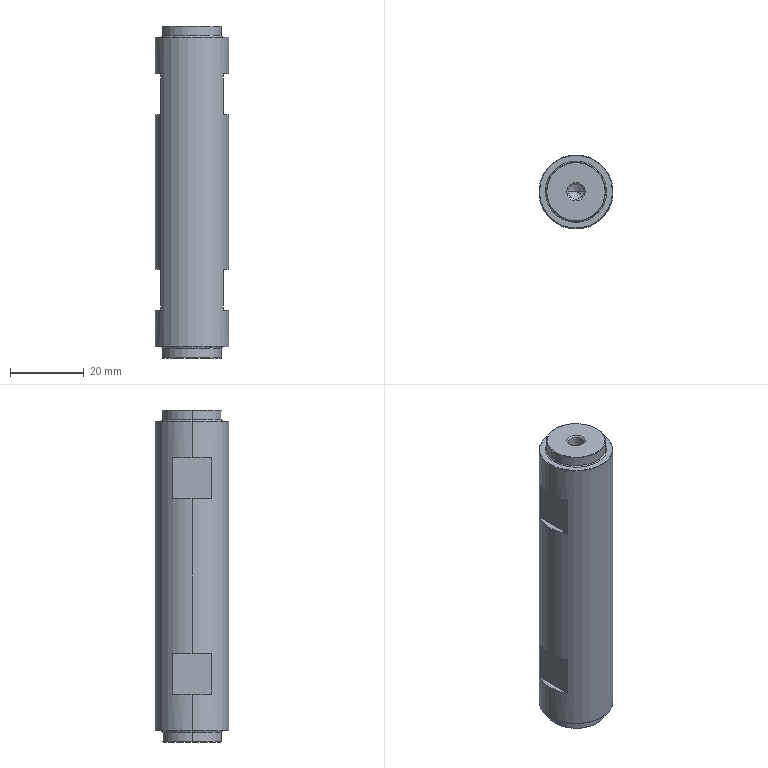Part | SolidWorks | features BaseBody 1 | 1 solid | 46 faces | box 20 x 20 x 90 mm | volume 26843 mm3 | cone 16 | plane 16 | cylinder 10 | spline 4 | commonest cylinder face diameters 4.134 x4 16 x4 20 x2
STEP:
#1=CARTESIAN_POINT('',(8.,0.,-2.7));
#2=VERTEX_POINT('',#1);
#3=CARTESIAN_POINT('',(-8.,0.,-2.7));
#4=VERTEX_POINT('',#3);
#5=CARTESIAN_POINT('',(0.,0.,-2.7));
#6=DIRECTION('',(0.,0.,1.));
#7=DIRECTION('',(-1.,0.,0.));
#8=AXIS2_PLACEMENT_3D('',#5,#6,#7);
#9=CIRCLE('',#8,8.);
#10=EDGE_CURVE('',#2,#4,#9,.T.);
#11=ORIENTED_EDGE('',*,*,#10,.F.);
#12=CARTESIAN_POINT('',(8.3,0.,-3.));
#13=VERTEX_POINT('',#12);
#14=CARTESIAN_POINT('',(8.3,0.,-2.7));
#15=DIRECTION('',(0.,-1.,0.));
#16=DIRECTION('',(1.,0.,0.));
#17=AXIS2_PLACEMENT_3D('',#14,#15,#16);
#18=CIRCLE('',#17,0.3);
#19=EDGE_CURVE('',#2,#13,#18,.T.);
#20=ORIENTED_EDGE('',*,*,#19,.T.);
#21=CARTESIAN_POINT('',(-8.3,0.,-3.));
#22=VERTEX_POINT('',#21);
#23=CARTESIAN_POINT('',(8.3,0.,-3.));
#24=CARTESIAN_POINT('',(8.3,16.6,-3.));
#25=CARTESIAN_POINT('',(-8.3,16.6,-3.));
#26=CARTESIAN_POINT('',(-8.3,0.,-3.));
#27=(BOUNDED_CURVE()B_SPLINE_CURVE(3,(#23,#24,#25,#26),.UNSPECIFIED.,.F.,.F.)B_SPLINE_CURVE_WITH_KNOTS((4,4),(0.5,1.),.UNSPECIFIED.)CURVE()GEOMETRIC_REPRESENTATION_ITEM()RATIONAL_B_SPLINE_CURVE((1.,0.3333,0.3333,1.))REPRESENTATION_ITEM(''));
#28=EDGE_CURVE('',#13,#22,#27,.T.);
#29=ORIENTED_EDGE('',*,*,#28,.T.);
#30=CARTESIAN_POINT('',(-8.3,0.,-2.7));
#31=DIRECTION('',(0.,1.,0.));
#32=DIRECTION('',(-1.,0.,0.));
#33=AXIS2_PLACEMENT_3D('',#30,#31,#32);
#34=CIRCLE('',#33,0.3);
#35=EDGE_CURVE('',#4,#22,#34,.T.);
#36=ORIENTED_EDGE('',*,*,#35,.F.);
#37=EDGE_LOOP('',(#11,#20,#29,#36));
#38=FACE_OUTER_BOUND('',#37,.T.);
#39=CARTESIAN_POINT('',(-8.,0.,-2.7));
#40=CARTESIAN_POINT('',(-8.,16.,-2.7));
#41=CARTESIAN_POINT('',(8.,16.,-2.7));
#42=CARTESIAN_POINT('',(8.,0.,-2.7));
#43=CARTESIAN_POINT('',(-8.,0.,-2.876));
#44=CARTESIAN_POINT('',(-8.,16.,-2.876));
#45=CARTESIAN_POINT('',(8.,16.,-2.876));
#46=CARTESIAN_POINT('',(8.,0.,-2.876));
#47=CARTESIAN_POINT('',(-8.124,0.,-3.));
#48=CARTESIAN_POINT('',(-8.124,16.249,-3.));
#49=CARTESIAN_POINT('',(8.124,16.249,-3.));
#50=CARTESIAN_POINT('',(8.124,0.,-3.));
#51=CARTESIAN_POINT('',(-8.3,0.,-3.));
#52=CARTESIAN_POINT('',(-8.3,16.6,-3.));
#53=CARTESIAN_POINT('',(8.3,16.6,-3.));
#54=CARTESIAN_POINT('',(8.3,0.,-3.));
#55=(BOUNDED_SURFACE()B_SPLINE_SURFACE(3,3,((#39,#40,#41,#42),(#43,#44,#45,#46),(#47,#48,#49,#50),(#51,#52,#53,#54)),.UNSPECIFIED.,.F.,.F.,.F.)B_SPLINE_SURFACE_WITH_KNOTS((4,4),(4,4),(0.,1.),(0.,1.),.UNSPECIFIED.)GEOMETRIC_REPRESENTATION_ITEM()RATIONAL_B_SPLINE_SURFACE(((1.,0.3333,0.3333,1.),(0.8047,0.2682,0.2682,0.8047),(0.8047,0.2682,0.2682,0.8047),(1.,0.3333,0.3333,1.)))REPRESENTATION_ITEM('')SURFACE());
#56=ADVANCED_FACE('',(#38),#55,.F.);
#57=CARTESIAN_POINT('',(-8.3,0.,-87.));
#58=VERTEX_POINT('',#57);
#59=CARTESIAN_POINT('',(8.3,0.,-87.));
#60=VERTEX_POINT('',#59);
#61=CARTESIAN_POINT('',(-8.3,0.,-87.));
#62=CARTESIAN_POINT('',(-8.3,16.6,-87.));
#63=CARTESIAN_POINT('',(8.3,16.6,-87.));
#64=CARTESIAN_POINT('',(8.3,0.,-87.));
#65=(BOUNDED_CURVE()B_SPLINE_CURVE(3,(#61,#62,#63,#64),.UNSPECIFIED.,.F.,.T.)B_SPLINE_CURVE_WITH_KNOTS((4,4),(0.,0.5),.UNSPECIFIED.)CURVE()GEOMETRIC_REPRESENTATION_ITEM()RATIONAL_B_SPLINE_CURVE((1.,0.3333,0.3333,1.))REPRESENTATION_ITEM(''));
#66=EDGE_CURVE('',#58,#60,#65,.T.);
#67=ORIENTED_EDGE('',*,*,#66,.T.);
#68=CARTESIAN_POINT('',(8.,0.,-87.3));
#69=VERTEX_POINT('',#68);
#70=CARTESIAN_POINT('',(8.3,0.,-87.3));
#71=DIRECTION('',(0.,-1.,0.));
#72=DIRECTION('',(1.,0.,0.));
#73=AXIS2_PLACEMENT_3D('',#70,#71,#72);
#74=CIRCLE('',#73,0.3);
#75=EDGE_CURVE('',#60,#69,#74,.T.);
#76=ORIENTED_EDGE('',*,*,#75,.T.);
#77=CARTESIAN_POINT('',(-8.,0.,-87.3));
#78=VERTEX_POINT('',#77);
#79=CARTESIAN_POINT('',(0.,0.,-87.3));
#80=DIRECTION('',(0.,0.,-1.));
#81=DIRECTION('',(-1.,0.,0.));
#82=AXIS2_PLACEMENT_3D('',#79,#80,#81);
#83=CIRCLE('',#82,8.);
#84=EDGE_CURVE('',#78,#69,#83,.T.);
#85=ORIENTED_EDGE('',*,*,#84,.F.);
#86=CARTESIAN_POINT('',(-8.3,0.,-87.3));
#87=DIRECTION('',(0.,1.,0.));
#88=DIRECTION('',(-1.,0.,0.));
#89=AXIS2_PLACEMENT_3D('',#86,#87,#88);
#90=CIRCLE('',#89,0.3);
#91=EDGE_CURVE('',#58,#78,#90,.T.);
#92=ORIENTED_EDGE('',*,*,#91,.F.);
#93=EDGE_LOOP('',(#67,#76,#85,#92));
#94=FACE_OUTER_BOUND('',#93,.T.);
#95=CARTESIAN_POINT('',(-8.3,0.,-87.));
#96=CARTESIAN_POINT('',(-8.3,16.6,-87.));
#97=CARTESIAN_POINT('',(8.3,16.6,-87.));
#98=CARTESIAN_POINT('',(8.3,0.,-87.));
#99=CARTESIAN_POINT('',(-8.124,0.,-87.));
#100=CARTESIAN_POINT('',(-8.124,16.249,-87.));
#101=CARTESIAN_POINT('',(8.124,16.249,-87.));
#102=CARTESIAN_POINT('',(8.124,0.,-87.));
#103=CARTESIAN_POINT('',(-8.,0.,-87.124));
#104=CARTESIAN_POINT('',(-8.,16.,-87.124));
#105=CARTESIAN_POINT('',(8.,16.,-87.124));
#106=CARTESIAN_POINT('',(8.,0.,-87.124));
#107=CARTESIAN_POINT('',(-8.,0.,-87.3));
#108=CARTESIAN_POINT('',(-8.,16.,-87.3));
#109=CARTESIAN_POINT('',(8.,16.,-87.3));
#110=CARTESIAN_POINT('',(8.,0.,-87.3));
#111=(BOUNDED_SURFACE()B_SPLINE_SURFACE(3,3,((#95,#96,#97,#98),(#99,#100,#101,#102),(#103,#104,#105,#106),(#107,#108,#109,#110)),.UNSPECIFIED.,.F.,.F.,.F.)B_SPLINE_SURFACE_WITH_KNOTS((4,4),(4,4),(0.,1.),(0.,1.),.UNSPECIFIED.)GEOMETRIC_REPRESENTATION_ITEM()RATIONAL_B_SPLINE_SURFACE(((1.,0.3333,0.3333,1.),(0.8047,0.2682,0.2682,0.8047),(0.8047,0.2682,0.2682,0.8047),(1.,0.3333,0.3333,1.)))REPRESENTATION_ITEM('')SURFACE());
#112=ADVANCED_FACE('',(#94),#111,.F.);
#113=CARTESIAN_POINT('',(10.,0.,-86.9));
#114=VERTEX_POINT('',#113);
#115=CARTESIAN_POINT('',(-10.,0.,-86.9));
#116=VERTEX_POINT('',#115);
#117=CARTESIAN_POINT('',(0.,0.,-86.9));
#118=DIRECTION('',(0.,0.,1.));
#119=DIRECTION('',(1.,0.,0.));
#120=AXIS2_PLACEMENT_3D('',#117,#118,#119);
#121=CIRCLE('',#120,10.);
#122=EDGE_CURVE('',#114,#116,#121,.T.);
#123=ORIENTED_EDGE('',*,*,#122,.T.);
#124=CARTESIAN_POINT('',(-10.,0.,-77.));
#125=VERTEX_POINT('',#124);
#126=CARTESIAN_POINT('',(-10.,0.,-90.));
#127=DIRECTION('',(0.,0.,1.));
#128=VECTOR('',#127,1000.);
#129=LINE('',#126,#128);
#130=EDGE_CURVE('',#116,#125,#129,.T.);
#131=ORIENTED_EDGE('',*,*,#130,.T.);
#132=CARTESIAN_POINT('',(-8.5,5.268,-77.));
#133=VERTEX_POINT('',#132);
#134=CARTESIAN_POINT('',(0.,0.,-77.));
#135=DIRECTION('',(0.,0.,-1.));
#136=DIRECTION('',(1.,0.,0.));
#137=AXIS2_PLACEMENT_3D('',#134,#135,#136);
#138=CIRCLE('',#137,10.);
#139=EDGE_CURVE('',#125,#133,#138,.T.);
#140=ORIENTED_EDGE('',*,*,#139,.T.);
#141=CARTESIAN_POINT('',(-8.5,5.268,-66.));
#142=VERTEX_POINT('',#141);
#143=CARTESIAN_POINT('',(-8.5,5.268,-90.));
#144=DIRECTION('',(0.,0.,1.));
#145=VECTOR('',#144,1000.);
#146=LINE('',#143,#145);
#147=EDGE_CURVE('',#133,#142,#146,.T.);
#148=ORIENTED_EDGE('',*,*,#147,.T.);
#149=CARTESIAN_POINT('',(-10.,0.,-66.));
#150=VERTEX_POINT('',#149);
#151=CARTESIAN_POINT('',(0.,0.,-66.));
#152=DIRECTION('',(0.,0.,1.));
#153=DIRECTION('',(1.,0.,0.));
#154=AXIS2_PLACEMENT_3D('',#151,#152,#153);
#155=CIRCLE('',#154,10.);
#156=EDGE_CURVE('',#142,#150,#155,.T.);
#157=ORIENTED_EDGE('',*,*,#156,.T.);
#158=CARTESIAN_POINT('',(-10.,0.,-24.));
#159=VERTEX_POINT('',#158);
#160=CARTESIAN_POINT('',(-10.,0.,-90.));
#161=DIRECTION('',(0.,0.,1.));
#162=VECTOR('',#161,1000.);
#163=LINE('',#160,#162);
#164=EDGE_CURVE('',#150,#159,#163,.T.);
#165=ORIENTED_EDGE('',*,*,#164,.T.);
#166=CARTESIAN_POINT('',(-8.5,5.268,-24.));
#167=VERTEX_POINT('',#166);
#168=CARTESIAN_POINT('',(0.,0.,-24.));
#169=DIRECTION('',(0.,0.,-1.));
#170=DIRECTION('',(1.,0.,0.));
#171=AXIS2_PLACEMENT_3D('',#168,#169,#170);
#172=CIRCLE('',#171,10.);
#173=EDGE_CURVE('',#159,#167,#172,.T.);
#174=ORIENTED_EDGE('',*,*,#173,.T.);
#175=CARTESIAN_POINT('',(-8.5,5.268,-13.));
#176=VERTEX_POINT('',#175);
#177=CARTESIAN_POINT('',(-8.5,5.268,-90.));
#178=DIRECTION('',(0.,0.,1.));
#179=VECTOR('',#178,1000.);
#180=LINE('',#177,#179);
#181=EDGE_CURVE('',#167,#176,#180,.T.);
#182=ORIENTED_EDGE('',*,*,#181,.T.);
#183=CARTESIAN_POINT('',(-10.,0.,-13.));
#184=VERTEX_POINT('',#183);
#185=CARTESIAN_POINT('',(0.,0.,-13.));
#186=DIRECTION('',(0.,0.,1.));
#187=DIRECTION('',(1.,0.,0.));
#188=AXIS2_PLACEMENT_3D('',#185,#186,#187);
#189=CIRCLE('',#188,10.);
#190=EDGE_CURVE('',#176,#184,#189,.T.);
#191=ORIENTED_EDGE('',*,*,#190,.T.);
#192=CARTESIAN_POINT('',(-10.,0.,-3.1));
#193=VERTEX_POINT('',#192);
#194=CARTESIAN_POINT('',(-10.,0.,-90.));
#195=DIRECTION('',(0.,0.,1.));
#196=VECTOR('',#195,1000.);
#197=LINE('',#194,#196);
#198=EDGE_CURVE('',#184,#193,#197,.T.);
#199=ORIENTED_EDGE('',*,*,#198,.T.);
#200=CARTESIAN_POINT('',(10.,0.,-3.1));
#201=VERTEX_POINT('',#200);
#202=CARTESIAN_POINT('',(0.,0.,-3.1));
#203=DIRECTION('',(0.,0.,-1.));
#204=DIRECTION('',(1.,0.,0.));
#205=AXIS2_PLACEMENT_3D('',#202,#203,#204);
#206=CIRCLE('',#205,10.);
#207=EDGE_CURVE('',#193,#201,#206,.T.);
#208=ORIENTED_EDGE('',*,*,#207,.T.);
#209=CARTESIAN_POINT('',(10.,0.,-13.));
#210=VERTEX_POINT('',#209);
#211=CARTESIAN_POINT('',(10.,0.,-90.));
#212=DIRECTION('',(0.,0.,1.));
#213=VECTOR('',#212,1000.);
#214=LINE('',#211,#213);
#215=EDGE_CURVE('',#210,#201,#214,.T.);
#216=ORIENTED_EDGE('',*,*,#215,.F.);
#217=CARTESIAN_POINT('',(8.5,5.268,-13.));
#218=VERTEX_POINT('',#217);
#219=CARTESIAN_POINT('',(0.,0.,-13.));
#220=DIRECTION('',(0.,0.,1.));
#221=DIRECTION('',(1.,0.,0.));
#222=AXIS2_PLACEMENT_3D('',#219,#220,#221);
#223=CIRCLE('',#222,10.);
#224=EDGE_CURVE('',#210,#218,#223,.T.);
#225=ORIENTED_EDGE('',*,*,#224,.T.);
#226=CARTESIAN_POINT('',(8.5,5.268,-24.));
#227=VERTEX_POINT('',#226);
#228=CARTESIAN_POINT('',(8.5,5.268,-90.));
#229=DIRECTION('',(0.,0.,-1.));
#230=VECTOR('',#229,1000.);
#231=LINE('',#228,#230);
#232=EDGE_CURVE('',#218,#227,#231,.T.);
#233=ORIENTED_EDGE('',*,*,#232,.T.);
#234=CARTESIAN_POINT('',(10.,0.,-24.));
#235=VERTEX_POINT('',#234);
#236=CARTESIAN_POINT('',(0.,0.,-24.));
#237=DIRECTION('',(0.,0.,-1.));
#238=DIRECTION('',(1.,0.,0.));
#239=AXIS2_PLACEMENT_3D('',#236,#237,#238);
#240=CIRCLE('',#239,10.);
#241=EDGE_CURVE('',#227,#235,#240,.T.);
#242=ORIENTED_EDGE('',*,*,#241,.T.);
#243=CARTESIAN_POINT('',(10.,0.,-66.));
#244=VERTEX_POINT('',#243);
#245=CARTESIAN_POINT('',(10.,0.,-90.));
#246=DIRECTION('',(0.,0.,1.));
#247=VECTOR('',#246,1000.);
#248=LINE('',#245,#247);
#249=EDGE_CURVE('',#244,#235,#248,.T.);
#250=ORIENTED_EDGE('',*,*,#249,.F.);
#251=CARTESIAN_POINT('',(8.5,5.268,-66.));
#252=VERTEX_POINT('',#251);
#253=CARTESIAN_POINT('',(0.,0.,-66.));
#254=DIRECTION('',(0.,0.,1.));
#255=DIRECTION('',(1.,0.,0.));
#256=AXIS2_PLACEMENT_3D('',#253,#254,#255);
#257=CIRCLE('',#256,10.);
#258=EDGE_CURVE('',#244,#252,#257,.T.);
#259=ORIENTED_EDGE('',*,*,#258,.T.);
#260=CARTESIAN_POINT('',(8.5,5.268,-77.));
#261=VERTEX_POINT('',#260);
#262=CARTESIAN_POINT('',(8.5,5.268,-90.));
#263=DIRECTION('',(0.,0.,-1.));
#264=VECTOR('',#263,1000.);
#265=LINE('',#262,#264);
#266=EDGE_CURVE('',#252,#261,#265,.T.);
#267=ORIENTED_EDGE('',*,*,#266,.T.);
#268=CARTESIAN_POINT('',(10.,0.,-77.));
#269=VERTEX_POINT('',#268);
#270=CARTESIAN_POINT('',(0.,0.,-77.));
#271=DIRECTION('',(0.,0.,-1.));
#272=DIRECTION('',(1.,0.,0.));
#273=AXIS2_PLACEMENT_3D('',#270,#271,#272);
#274=CIRCLE('',#273,10.);
#275=EDGE_CURVE('',#261,#269,#274,.T.);
#276=ORIENTED_EDGE('',*,*,#275,.T.);
#277=CARTESIAN_POINT('',(10.,0.,-90.));
#278=DIRECTION('',(0.,0.,1.));
#279=VECTOR('',#278,1000.);
#280=LINE('',#277,#279);
#281=EDGE_CURVE('',#114,#269,#280,.T.);
#282=ORIENTED_EDGE('',*,*,#281,.F.);
#283=EDGE_LOOP('',(#123,#131,#140,#148,#157,#165,#174,#182,#191,#199,#208,#216,#225,#233,#242,#250,#259,#267,#276,#282));
#284=FACE_OUTER_BOUND('',#283,.T.);
#285=CARTESIAN_POINT('',(0.,0.,-90.));
#286=DIRECTION('',(0.,0.,1.));
#287=DIRECTION('',(1.,0.,0.));
#288=AXIS2_PLACEMENT_3D('',#285,#286,#287);
#289=CYLINDRICAL_SURFACE('',#288,10.);
#290=ADVANCED_FACE('',(#284),#289,.T.);
#291=CARTESIAN_POINT('',(-9.9,0.,-3.));
#292=VERTEX_POINT('',#291);
#293=CARTESIAN_POINT('',(9.9,0.,-3.));
#294=VERTEX_POINT('',#293);
#295=CARTESIAN_POINT('',(0.,0.,-3.));
#296=DIRECTION('',(0.,0.,-1.));
#297=DIRECTION('',(-1.,0.,0.));
#298=AXIS2_PLACEMENT_3D('',#295,#296,#297);
#299=CIRCLE('',#298,9.9);
#300=EDGE_CURVE('',#292,#294,#299,.T.);
#301=ORIENTED_EDGE('',*,*,#300,.T.);
#302=CARTESIAN_POINT('',(10.,0.,-3.1));
#303=DIRECTION('',(0.7071,0.,-0.7071));
#304=VECTOR('',#303,1000.);
#305=LINE('',#302,#304);
#306=EDGE_CURVE('',#294,#201,#305,.T.);
#307=ORIENTED_EDGE('',*,*,#306,.T.);
#308=ORIENTED_EDGE('',*,*,#207,.F.);
#309=CARTESIAN_POINT('',(-10.,0.,-3.1));
#310=DIRECTION('',(-0.7071,0.,-0.7071));
#311=VECTOR('',#310,1000.);
#312=LINE('',#309,#311);
#313=EDGE_CURVE('',#292,#193,#312,.T.);
#314=ORIENTED_EDGE('',*,*,#313,.F.);
#315=EDGE_LOOP('',(#301,#307,#308,#314));
#316=FACE_OUTER_BOUND('',#315,.T.);
#317=CARTESIAN_POINT('',(0.,0.,-3.1));
#318=DIRECTION('',(0.,0.,-1.));
#319=DIRECTION('',(-1.,0.,0.));
#320=AXIS2_PLACEMENT_3D('',#317,#318,#319);
#321=CONICAL_SURFACE('',#320,10.,0.7854);
#322=ADVANCED_FACE('',(#316),#321,.T.);
#323=CARTESIAN_POINT('',(9.9,0.,-87.));
#324=VERTEX_POINT('',#323);
#325=CARTESIAN_POINT('',(-9.9,0.,-87.));
#326=VERTEX_POINT('',#325);
#327=CARTESIAN_POINT('',(0.,0.,-87.));
#328=DIRECTION('',(0.,0.,1.));
#329=DIRECTION('',(1.,0.,0.));
#330=AXIS2_PLACEMENT_3D('',#327,#328,#329);
#331=CIRCLE('',#330,9.9);
#332=EDGE_CURVE('',#324,#326,#331,.T.);
#333=ORIENTED_EDGE('',*,*,#332,.T.);
#334=CARTESIAN_POINT('',(-10.,0.,-86.9));
#335=DIRECTION('',(-0.7071,0.,0.7071));
#336=VECTOR('',#335,1000.);
#337=LINE('',#334,#336);
#338=EDGE_CURVE('',#326,#116,#337,.T.);
#339=ORIENTED_EDGE('',*,*,#338,.T.);
#340=ORIENTED_EDGE('',*,*,#122,.F.);
#341=CARTESIAN_POINT('',(10.,0.,-86.9));
#342=DIRECTION('',(0.7071,0.,0.7071));
#343=VECTOR('',#342,1000.);
#344=LINE('',#341,#343);
#345=EDGE_CURVE('',#324,#114,#344,.T.);
#346=ORIENTED_EDGE('',*,*,#345,.F.);
#347=EDGE_LOOP('',(#333,#339,#340,#346));
#348=FACE_OUTER_BOUND('',#347,.T.);
#349=CARTESIAN_POINT('',(0.,0.,-86.9));
#350=DIRECTION('',(0.,0.,1.));
#351=DIRECTION('',(1.,0.,0.));
#352=AXIS2_PLACEMENT_3D('',#349,#350,#351);
#353=CONICAL_SURFACE('',#352,10.,0.7854);
#354=ADVANCED_FACE('',(#348),#353,.T.);
#355=ORIENTED_EDGE('',*,*,#10,.T.);
#356=CARTESIAN_POINT('',(-8.,0.,-0.1));
#357=VERTEX_POINT('',#356);
#358=CARTESIAN_POINT('',(-8.,0.,-90.));
#359=DIRECTION('',(0.,0.,1.));
#360=VECTOR('',#359,1000.);
#361=LINE('',#358,#360);
#362=EDGE_CURVE('',#4,#357,#361,.T.);
#363=ORIENTED_EDGE('',*,*,#362,.T.);
#364=CARTESIAN_POINT('',(8.,0.,-0.1));
#365=VERTEX_POINT('',#364);
#366=CARTESIAN_POINT('',(0.,0.,-0.1));
#367=DIRECTION('',(0.,0.,-1.));
#368=DIRECTION('',(1.,0.,0.));
#369=AXIS2_PLACEMENT_3D('',#366,#367,#368);
#370=CIRCLE('',#369,8.);
#371=EDGE_CURVE('',#357,#365,#370,.T.);
#372=ORIENTED_EDGE('',*,*,#371,.T.);
#373=CARTESIAN_POINT('',(8.,0.,-90.));
#374=DIRECTION('',(0.,0.,1.));
#375=VECTOR('',#374,1000.);
#376=LINE('',#373,#375);
#377=EDGE_CURVE('',#2,#365,#376,.T.);
#378=ORIENTED_EDGE('',*,*,#377,.F.);
#379=EDGE_LOOP('',(#355,#363,#372,#378));
#380=FACE_OUTER_BOUND('',#379,.T.);
#381=CARTESIAN_POINT('',(0.,0.,-90.));
#382=DIRECTION('',(0.,0.,1.));
#383=DIRECTION('',(1.,0.,0.));
#384=AXIS2_PLACEMENT_3D('',#381,#382,#383);
#385=CYLINDRICAL_SURFACE('',#384,8.);
#386=ADVANCED_FACE('',(#380),#385,.T.);
#387=CARTESIAN_POINT('',(8.,0.,-89.9));
#388=VERTEX_POINT('',#387);
#389=CARTESIAN_POINT('',(-8.,0.,-89.9));
#390=VERTEX_POINT('',#389);
#391=CARTESIAN_POINT('',(0.,0.,-89.9));
#392=DIRECTION('',(0.,0.,1.));
#393=DIRECTION('',(1.,0.,0.));
#394=AXIS2_PLACEMENT_3D('',#391,#392,#393);
#395=CIRCLE('',#394,8.);
#396=EDGE_CURVE('',#388,#390,#395,.T.);
#397=ORIENTED_EDGE('',*,*,#396,.T.);
#398=CARTESIAN_POINT('',(-8.,0.,-90.));
#399=DIRECTION('',(0.,0.,1.));
#400=VECTOR('',#399,1000.);
#401=LINE('',#398,#400);
#402=EDGE_CURVE('',#390,#78,#401,.T.);
#403=ORIENTED_EDGE('',*,*,#402,.T.);
#404=ORIENTED_EDGE('',*,*,#84,.T.);
#405=CARTESIAN_POINT('',(8.,0.,-90.));
#406=DIRECTION('',(0.,0.,1.));
#407=VECTOR('',#406,1000.);
#408=LINE('',#405,#407);
#409=EDGE_CURVE('',#388,#69,#408,.T.);
#410=ORIENTED_EDGE('',*,*,#409,.F.);
#411=EDGE_LOOP('',(#397,#403,#404,#410));
#412=FACE_OUTER_BOUND('',#411,.T.);
#413=CARTESIAN_POINT('',(0.,0.,-90.));
#414=DIRECTION('',(0.,0.,1.));
#415=DIRECTION('',(1.,0.,0.));
#416=AXIS2_PLACEMENT_3D('',#413,#414,#415);
#417=CYLINDRICAL_SURFACE('',#416,8.);
#418=ADVANCED_FACE('',(#412),#417,.T.);
#419=CARTESIAN_POINT('',(-7.9,0.,0.));
#420=VERTEX_POINT('',#419);
#421=CARTESIAN_POINT('',(7.9,0.,0.));
#422=VERTEX_POINT('',#421);
#423=CARTESIAN_POINT('',(0.,0.,0.));
#424=DIRECTION('',(0.,0.,-1.));
#425=DIRECTION('',(-1.,0.,0.));
#426=AXIS2_PLACEMENT_3D('',#423,#424,#425);
#427=CIRCLE('',#426,7.9);
#428=EDGE_CURVE('',#420,#422,#427,.T.);
#429=ORIENTED_EDGE('',*,*,#428,.T.);
#430=CARTESIAN_POINT('',(8.,0.,-0.1));
#431=DIRECTION('',(0.7071,0.,-0.7071));
#432=VECTOR('',#431,1000.);
#433=LINE('',#430,#432);
#434=EDGE_CURVE('',#422,#365,#433,.T.);
#435=ORIENTED_EDGE('',*,*,#434,.T.);
#436=ORIENTED_EDGE('',*,*,#371,.F.);
#437=CARTESIAN_POINT('',(-8.,0.,-0.1));
#438=DIRECTION('',(-0.7071,0.,-0.7071));
#439=VECTOR('',#438,1000.);
#440=LINE('',#437,#439);
#441=EDGE_CURVE('',#420,#357,#440,.T.);
#442=ORIENTED_EDGE('',*,*,#441,.F.);
#443=EDGE_LOOP('',(#429,#435,#436,#442));
#444=FACE_OUTER_BOUND('',#443,.T.);
#445=CARTESIAN_POINT('',(0.,0.,-0.1));
#446=DIRECTION('',(0.,0.,-1.));
#447=DIRECTION('',(-1.,0.,0.));
#448=AXIS2_PLACEMENT_3D('',#445,#446,#447);
#449=CONICAL_SURFACE('',#448,8.,0.7854);
#450=ADVANCED_FACE('',(#444),#449,.T.);
#451=CARTESIAN_POINT('',(7.9,0.,-90.));
#452=VERTEX_POINT('',#451);
#453=CARTESIAN_POINT('',(-7.9,0.,-90.));
#454=VERTEX_POINT('',#453);
#455=CARTESIAN_POINT('',(0.,0.,-90.));
#456=DIRECTION('',(0.,0.,1.));
#457=DIRECTION('',(1.,0.,0.));
#458=AXIS2_PLACEMENT_3D('',#455,#456,#457);
#459=CIRCLE('',#458,7.9);
#460=EDGE_CURVE('',#452,#454,#459,.T.);
#461=ORIENTED_EDGE('',*,*,#460,.T.);
#462=CARTESIAN_POINT('',(-8.,0.,-89.9));
#463=DIRECTION('',(-0.7071,0.,0.7071));
#464=VECTOR('',#463,1000.);
#465=LINE('',#462,#464);
#466=EDGE_CURVE('',#454,#390,#465,.T.);
#467=ORIENTED_EDGE('',*,*,#466,.T.);
#468=ORIENTED_EDGE('',*,*,#396,.F.);
#469=CARTESIAN_POINT('',(8.,0.,-89.9));
#470=DIRECTION('',(0.7071,0.,0.7071));
#471=VECTOR('',#470,1000.);
#472=LINE('',#469,#471);
#473=EDGE_CURVE('',#452,#388,#472,.T.);
#474=ORIENTED_EDGE('',*,*,#473,.F.);
#475=EDGE_LOOP('',(#461,#467,#468,#474));
#476=FACE_OUTER_BOUND('',#475,.T.);
#477=CARTESIAN_POINT('',(0.,0.,-89.9));
#478=DIRECTION('',(0.,0.,1.));
#479=DIRECTION('',(1.,0.,0.));
#480=AXIS2_PLACEMENT_3D('',#477,#478,#479);
#481=CONICAL_SURFACE('',#480,8.,0.7854);
#482=ADVANCED_FACE('',(#476),#481,.T.);
#483=CARTESIAN_POINT('',(-2.067,0.,-0.433));
#484=VERTEX_POINT('',#483);
#485=CARTESIAN_POINT('',(2.067,0.,-0.433));
#486=VERTEX_POINT('',#485);
#487=CARTESIAN_POINT('',(0.,0.,-0.433));
#488=DIRECTION('',(0.,0.,1.));
#489=DIRECTION('',(1.,0.,0.));
#490=AXIS2_PLACEMENT_3D('',#487,#488,#489);
#491=CIRCLE('',#490,2.067);
#492=EDGE_CURVE('',#484,#486,#491,.T.);
#493=ORIENTED_EDGE('',*,*,#492,.F.);
#494=CARTESIAN_POINT('',(-2.5,0.,0.));
#495=VERTEX_POINT('',#494);
#496=CARTESIAN_POINT('',(-2.5,0.,0.));
#497=DIRECTION('',(-0.7071,0.,0.7071));
#498=VECTOR('',#497,1000.);
#499=LINE('',#496,#498);
#500=EDGE_CURVE('',#484,#495,#499,.T.);
#501=ORIENTED_EDGE('',*,*,#500,.T.);
#502=CARTESIAN_POINT('',(2.5,0.,0.));
#503=VERTEX_POINT('',#502);
#504=CARTESIAN_POINT('',(0.,0.,0.));
#505=DIRECTION('',(0.,0.,1.));
#506=DIRECTION('',(1.,0.,0.));
#507=AXIS2_PLACEMENT_3D('',#504,#505,#506);
#508=CIRCLE('',#507,2.5);
#509=EDGE_CURVE('',#495,#503,#508,.T.);
#510=ORIENTED_EDGE('',*,*,#509,.T.);
#511=CARTESIAN_POINT('',(2.5,0.,0.));
#512=DIRECTION('',(0.7071,0.,0.7071));
#513=VECTOR('',#512,1000.);
#514=LINE('',#511,#513);
#515=EDGE_CURVE('',#486,#503,#514,.T.);
#516=ORIENTED_EDGE('',*,*,#515,.F.);
#517=EDGE_LOOP('',(#493,#501,#510,#516));
#518=FACE_OUTER_BOUND('',#517,.T.);
#519=CARTESIAN_POINT('',(0.,0.,0.));
#520=DIRECTION('',(0.,0.,1.));
#521=DIRECTION('',(1.,0.,0.));
#522=AXIS2_PLACEMENT_3D('',#519,#520,#521);
#523=CONICAL_SURFACE('',#522,2.5,0.7854);
#524=ADVANCED_FACE('',(#518),#523,.F.);
#525=CARTESIAN_POINT('',(2.067,0.,-89.567));
#526=VERTEX_POINT('',#525);
#527=CARTESIAN_POINT('',(-2.067,0.,-89.567));
#528=VERTEX_POINT('',#527);
#529=CARTESIAN_POINT('',(0.,0.,-89.567));
#530=DIRECTION('',(0.,0.,-1.));
#531=DIRECTION('',(-1.,0.,0.));
#532=AXIS2_PLACEMENT_3D('',#529,#530,#531);
#533=CIRCLE('',#532,2.067);
#534=EDGE_CURVE('',#526,#528,#533,.T.);
#535=ORIENTED_EDGE('',*,*,#534,.F.);
#536=CARTESIAN_POINT('',(2.5,0.,-90.));
#537=VERTEX_POINT('',#536);
#538=CARTESIAN_POINT('',(2.5,0.,-90.));
#539=DIRECTION('',(0.7071,0.,-0.7071));
#540=VECTOR('',#539,1000.);
#541=LINE('',#538,#540);
#542=EDGE_CURVE('',#526,#537,#541,.T.);
#543=ORIENTED_EDGE('',*,*,#542,.T.);
#544=CARTESIAN_POINT('',(-2.5,0.,-90.));
#545=VERTEX_POINT('',#544);
#546=CARTESIAN_POINT('',(0.,0.,-90.));
#547=DIRECTION('',(0.,0.,-1.));
#548=DIRECTION('',(-1.,0.,0.));
#549=AXIS2_PLACEMENT_3D('',#546,#547,#548);
#550=CIRCLE('',#549,2.5);
#551=EDGE_CURVE('',#537,#545,#550,.T.);
#552=ORIENTED_EDGE('',*,*,#551,.T.);
#553=CARTESIAN_POINT('',(-2.5,0.,-90.));
#554=DIRECTION('',(-0.7071,0.,-0.7071));
#555=VECTOR('',#554,1000.);
#556=LINE('',#553,#555);
#557=EDGE_CURVE('',#528,#545,#556,.T.);
#558=ORIENTED_EDGE('',*,*,#557,.F.);
#559=EDGE_LOOP('',(#535,#543,#552,#558));
#560=FACE_OUTER_BOUND('',#559,.T.);
#561=CARTESIAN_POINT('',(0.,0.,-90.));
#562=DIRECTION('',(0.,0.,-1.));
#563=DIRECTION('',(-1.,0.,0.));
#564=AXIS2_PLACEMENT_3D('',#561,#562,#563);
#565=CONICAL_SURFACE('',#564,2.5,0.7854);
#566=ADVANCED_FACE('',(#560),#565,.F.);
#567=CARTESIAN_POINT('',(-2.067,0.,-10.));
#568=VERTEX_POINT('',#567);
#569=CARTESIAN_POINT('',(2.067,0.,-10.));
#570=VERTEX_POINT('',#569);
#571=CARTESIAN_POINT('',(0.,0.,-10.));
#572=DIRECTION('',(0.,0.,1.));
#573=DIRECTION('',(1.,0.,0.));
#574=AXIS2_PLACEMENT_3D('',#571,#572,#573);
#575=CIRCLE('',#574,2.067);
#576=EDGE_CURVE('',#568,#570,#575,.T.);
#577=ORIENTED_EDGE('',*,*,#576,.F.);
#578=CARTESIAN_POINT('',(-2.067,0.,-11.193));
#579=DIRECTION('',(0.,0.,1.));
#580=VECTOR('',#579,1000.);
#581=LINE('',#578,#580);
#582=EDGE_CURVE('',#568,#484,#581,.T.);
#583=ORIENTED_EDGE('',*,*,#582,.T.);
#584=ORIENTED_EDGE('',*,*,#492,.T.);
#585=CARTESIAN_POINT('',(2.067,0.,-11.193));
#586=DIRECTION('',(0.,0.,1.));
#587=VECTOR('',#586,1000.);
#588=LINE('',#585,#587);
#589=EDGE_CURVE('',#570,#486,#588,.T.);
#590=ORIENTED_EDGE('',*,*,#589,.F.);
#591=EDGE_LOOP('',(#577,#583,#584,#590));
#592=FACE_OUTER_BOUND('',#591,.T.);
#593=CARTESIAN_POINT('',(0.,0.,-11.193));
#594=DIRECTION('',(0.,0.,1.));
#595=DIRECTION('',(1.,0.,0.));
#596=AXIS2_PLACEMENT_3D('',#593,#594,#595);
#597=CYLINDRICAL_SURFACE('',#596,2.067);
#598=ADVANCED_FACE('',(#592),#597,.F.);
#599=ORIENTED_EDGE('',*,*,#534,.T.);
#600=CARTESIAN_POINT('',(-2.067,0.,-80.));
#601=VERTEX_POINT('',#600);
#602=CARTESIAN_POINT('',(-2.067,0.,-90.));
#603=DIRECTION('',(0.,0.,1.));
#604=VECTOR('',#603,1000.);
#605=LINE('',#602,#604);
#606=EDGE_CURVE('',#528,#601,#605,.T.);
#607=ORIENTED_EDGE('',*,*,#606,.T.);
#608=CARTESIAN_POINT('',(2.067,0.,-80.));
#609=VERTEX_POINT('',#608);
#610=CARTESIAN_POINT('',(0.,0.,-80.));
#611=DIRECTION('',(0.,0.,-1.));
#612=DIRECTION('',(1.,0.,0.));
#613=AXIS2_PLACEMENT_3D('',#610,#611,#612);
#614=CIRCLE('',#613,2.067);
#615=EDGE_CURVE('',#609,#601,#614,.T.);
#616=ORIENTED_EDGE('',*,*,#615,.F.);
#617=CARTESIAN_POINT('',(2.067,0.,-90.));
#618=DIRECTION('',(0.,0.,1.));
#619=VECTOR('',#618,1000.);
#620=LINE('',#617,#619);
#621=EDGE_CURVE('',#526,#609,#620,.T.);
#622=ORIENTED_EDGE('',*,*,#621,.F.);
#623=EDGE_LOOP('',(#599,#607,#616,#622));
#624=FACE_OUTER_BOUND('',#623,.T.);
#625=CARTESIAN_POINT('',(0.,0.,-90.));
#626=DIRECTION('',(0.,0.,1.));
#627=DIRECTION('',(1.,0.,0.));
#628=AXIS2_PLACEMENT_3D('',#625,#626,#627);
#629=CYLINDRICAL_SURFACE('',#628,2.067);
#630=ADVANCED_FACE('',(#624),#629,.F.);
#631=CARTESIAN_POINT('',(0.,0.,-11.193));
#632=VERTEX_POINT('',#631);
#633=CARTESIAN_POINT('',(2.067,0.,-10.));
#634=DIRECTION('',(0.866,0.,0.5));
#635=VECTOR('',#634,1000.);
#636=LINE('',#633,#635);
#637=EDGE_CURVE('',#632,#570,#636,.T.);
#638=ORIENTED_EDGE('',*,*,#637,.F.);
#639=CARTESIAN_POINT('',(-2.067,0.,-10.));
#640=DIRECTION('',(-0.866,0.,0.5));
#641=VECTOR('',#640,1000.);
#642=LINE('',#639,#641);
#643=EDGE_CURVE('',#632,#568,#642,.T.);
#644=ORIENTED_EDGE('',*,*,#643,.T.);
#645=ORIENTED_EDGE('',*,*,#576,.T.);
#646=EDGE_LOOP('',(#638,#644,#645));
#647=FACE_OUTER_BOUND('',#646,.T.);
#648=CARTESIAN_POINT('',(0.,0.,-10.));
#649=DIRECTION('',(0.,0.,1.));
#650=DIRECTION('',(1.,0.,0.));
#651=AXIS2_PLACEMENT_3D('',#648,#649,#650);
#652=CONICAL_SURFACE('',#651,2.067,1.047);
#653=ADVANCED_FACE('',(#647),#652,.F.);
#654=CARTESIAN_POINT('',(0.,0.,-78.807));
#655=VERTEX_POINT('',#654);
#656=CARTESIAN_POINT('',(-2.067,0.,-80.));
#657=DIRECTION('',(-0.866,0.,-0.5));
#658=VECTOR('',#657,1000.);
#659=LINE('',#656,#658);
#660=EDGE_CURVE('',#655,#601,#659,.T.);
#661=ORIENTED_EDGE('',*,*,#660,.F.);
#662=CARTESIAN_POINT('',(2.067,0.,-80.));
#663=DIRECTION('',(0.866,0.,-0.5));
#664=VECTOR('',#663,1000.);
#665=LINE('',#662,#664);
#666=EDGE_CURVE('',#655,#609,#665,.T.);
#667=ORIENTED_EDGE('',*,*,#666,.T.);
#668=ORIENTED_EDGE('',*,*,#615,.T.);
#669=EDGE_LOOP('',(#661,#667,#668));
#670=FACE_OUTER_BOUND('',#669,.T.);
#671=CARTESIAN_POINT('',(0.,0.,-80.));
#672=DIRECTION('',(0.,0.,-1.));
#673=DIRECTION('',(-1.,0.,0.));
#674=AXIS2_PLACEMENT_3D('',#671,#672,#673);
#675=CONICAL_SURFACE('',#674,2.067,1.047);
#676=ADVANCED_FACE('',(#670),#675,.F.);
#677=ORIENTED_EDGE('',*,*,#130,.F.);
#678=CARTESIAN_POINT('',(0.,0.,-86.9));
#679=DIRECTION('',(0.,0.,1.));
#680=DIRECTION('',(1.,0.,0.));
#681=AXIS2_PLACEMENT_3D('',#678,#679,#680);
#682=CIRCLE('',#681,10.);
#683=EDGE_CURVE('',#116,#114,#682,.T.);
#684=ORIENTED_EDGE('',*,*,#683,.T.);
#685=ORIENTED_EDGE('',*,*,#281,.T.);
#686=CARTESIAN_POINT('',(8.5,-5.268,-77.));
#687=VERTEX_POINT('',#686);
#688=CARTESIAN_POINT('',(0.,0.,-77.));
#689=DIRECTION('',(0.,0.,-1.));
#690=DIRECTION('',(1.,0.,0.));
#691=AXIS2_PLACEMENT_3D('',#688,#689,#690);
#692=CIRCLE('',#691,10.);
#693=EDGE_CURVE('',#269,#687,#692,.T.);
#694=ORIENTED_EDGE('',*,*,#693,.T.);
#695=CARTESIAN_POINT('',(8.5,-5.268,-66.));
#696=VERTEX_POINT('',#695);
#697=CARTESIAN_POINT('',(8.5,-5.268,-90.));
#698=DIRECTION('',(0.,0.,1.));
#699=VECTOR('',#698,1000.);
#700=LINE('',#697,#699);
#701=EDGE_CURVE('',#687,#696,#700,.T.);
#702=ORIENTED_EDGE('',*,*,#701,.T.);
#703=CARTESIAN_POINT('',(0.,0.,-66.));
#704=DIRECTION('',(0.,0.,1.));
#705=DIRECTION('',(1.,0.,0.));
#706=AXIS2_PLACEMENT_3D('',#703,#704,#705);
#707=CIRCLE('',#706,10.);
#708=EDGE_CURVE('',#696,#244,#707,.T.);
#709=ORIENTED_EDGE('',*,*,#708,.T.);
#710=ORIENTED_EDGE('',*,*,#249,.T.);
#711=CARTESIAN_POINT('',(8.5,-5.268,-24.));
#712=VERTEX_POINT('',#711);
#713=CARTESIAN_POINT('',(0.,0.,-24.));
#714=DIRECTION('',(0.,0.,-1.));
#715=DIRECTION('',(1.,0.,0.));
#716=AXIS2_PLACEMENT_3D('',#713,#714,#715);
#717=CIRCLE('',#716,10.);
#718=EDGE_CURVE('',#235,#712,#717,.T.);
#719=ORIENTED_EDGE('',*,*,#718,.T.);
#720=CARTESIAN_POINT('',(8.5,-5.268,-13.));
#721=VERTEX_POINT('',#720);
#722=CARTESIAN_POINT('',(8.5,-5.268,-90.));
#723=DIRECTION('',(0.,0.,1.));
#724=VECTOR('',#723,1000.);
#725=LINE('',#722,#724);
#726=EDGE_CURVE('',#712,#721,#725,.T.);
#727=ORIENTED_EDGE('',*,*,#726,.T.);
#728=CARTESIAN_POINT('',(0.,0.,-13.));
#729=DIRECTION('',(0.,0.,1.));
#730=DIRECTION('',(1.,0.,0.));
#731=AXIS2_PLACEMENT_3D('',#728,#729,#730);
#732=CIRCLE('',#731,10.);
#733=EDGE_CURVE('',#721,#210,#732,.T.);
#734=ORIENTED_EDGE('',*,*,#733,.T.);
#735=ORIENTED_EDGE('',*,*,#215,.T.);
#736=CARTESIAN_POINT('',(0.,0.,-3.1));
#737=DIRECTION('',(0.,0.,-1.));
#738=DIRECTION('',(1.,0.,0.));
#739=AXIS2_PLACEMENT_3D('',#736,#737,#738);
#740=CIRCLE('',#739,10.);
#741=EDGE_CURVE('',#201,#193,#740,.T.);
#742=ORIENTED_EDGE('',*,*,#741,.T.);
#743=ORIENTED_EDGE('',*,*,#198,.F.);
#744=CARTESIAN_POINT('',(-8.5,-5.268,-13.));
#745=VERTEX_POINT('',#744);
#746=CARTESIAN_POINT('',(0.,0.,-13.));
#747=DIRECTION('',(0.,0.,1.));
#748=DIRECTION('',(1.,0.,0.));
#749=AXIS2_PLACEMENT_3D('',#746,#747,#748);
#750=CIRCLE('',#749,10.);
#751=EDGE_CURVE('',#184,#745,#750,.T.);
#752=ORIENTED_EDGE('',*,*,#751,.T.);
#753=CARTESIAN_POINT('',(-8.5,-5.268,-24.));
#754=VERTEX_POINT('',#753);
#755=CARTESIAN_POINT('',(-8.5,-5.268,-90.));
#756=DIRECTION('',(0.,0.,-1.));
#757=VECTOR('',#756,1000.);
#758=LINE('',#755,#757);
#759=EDGE_CURVE('',#745,#754,#758,.T.);
#760=ORIENTED_EDGE('',*,*,#759,.T.);
#761=CARTESIAN_POINT('',(0.,0.,-24.));
#762=DIRECTION('',(0.,0.,-1.));
#763=DIRECTION('',(1.,0.,0.));
#764=AXIS2_PLACEMENT_3D('',#761,#762,#763);
#765=CIRCLE('',#764,10.);
#766=EDGE_CURVE('',#754,#159,#765,.T.);
#767=ORIENTED_EDGE('',*,*,#766,.T.);
#768=ORIENTED_EDGE('',*,*,#164,.F.);
#769=CARTESIAN_POINT('',(-8.5,-5.268,-66.));
#770=VERTEX_POINT('',#769);
#771=CARTESIAN_POINT('',(0.,0.,-66.));
#772=DIRECTION('',(0.,0.,1.));
#773=DIRECTION('',(1.,0.,0.));
#774=AXIS2_PLACEMENT_3D('',#771,#772,#773);
#775=CIRCLE('',#774,10.);
#776=EDGE_CURVE('',#150,#770,#775,.T.);
#777=ORIENTED_EDGE('',*,*,#776,.T.);
#778=CARTESIAN_POINT('',(-8.5,-5.268,-77.));
#779=VERTEX_POINT('',#778);
#780=CARTESIAN_POINT('',(-8.5,-5.268,-90.));
#781=DIRECTION('',(0.,0.,-1.));
#782=VECTOR('',#781,1000.);
#783=LINE('',#780,#782);
#784=EDGE_CURVE('',#770,#779,#783,.T.);
#785=ORIENTED_EDGE('',*,*,#784,.T.);
#786=CARTESIAN_POINT('',(0.,0.,-77.));
#787=DIRECTION('',(0.,0.,-1.));
#788=DIRECTION('',(1.,0.,0.));
#789=AXIS2_PLACEMENT_3D('',#786,#787,#788);
#790=CIRCLE('',#789,10.);
#791=EDGE_CURVE('',#779,#125,#790,.T.);
#792=ORIENTED_EDGE('',*,*,#791,.T.);
#793=EDGE_LOOP('',(#677,#684,#685,#694,#702,#709,#710,#719,#727,#734,#735,#742,#743,#752,#760,#767,#768,#777,#785,#792));
#794=FACE_OUTER_BOUND('',#793,.T.);
#795=CARTESIAN_POINT('',(0.,0.,-90.));
#796=DIRECTION('',(0.,0.,1.));
#797=DIRECTION('',(1.,0.,0.));
#798=AXIS2_PLACEMENT_3D('',#795,#796,#797);
#799=CYLINDRICAL_SURFACE('',#798,10.);
#800=ADVANCED_FACE('',(#794),#799,.T.);
#801=CARTESIAN_POINT('',(-8.5,20.,-77.));
#802=DIRECTION('',(0.,1.,0.));
#803=VECTOR('',#802,1000.);
#804=LINE('',#801,#803);
#805=EDGE_CURVE('',#779,#133,#804,.T.);
#806=ORIENTED_EDGE('',*,*,#805,.T.);
#807=ORIENTED_EDGE('',*,*,#139,.F.);
#808=ORIENTED_EDGE('',*,*,#791,.F.);
#809=EDGE_LOOP('',(#806,#807,#808));
#810=FACE_OUTER_BOUND('',#809,.T.);
#811=CARTESIAN_POINT('',(-8.5,20.,-77.));
#812=DIRECTION('',(0.,0.,1.));
#813=DIRECTION('',(1.,0.,0.));
#814=AXIS2_PLACEMENT_3D('',#811,#812,#813);
#815=PLANE('',#814);
#816=ADVANCED_FACE('',(#810),#815,.T.);
#817=ORIENTED_EDGE('',*,*,#784,.F.);
#818=CARTESIAN_POINT('',(-8.5,20.,-66.));
#819=DIRECTION('',(0.,1.,0.));
#820=VECTOR('',#819,1000.);
#821=LINE('',#818,#820);
#822=EDGE_CURVE('',#770,#142,#821,.T.);
#823=ORIENTED_EDGE('',*,*,#822,.T.);
#824=ORIENTED_EDGE('',*,*,#147,.F.);
#825=ORIENTED_EDGE('',*,*,#805,.F.);
#826=EDGE_LOOP('',(#817,#823,#824,#825));
#827=FACE_OUTER_BOUND('',#826,.T.);
#828=CARTESIAN_POINT('',(-8.5,20.,-66.));
#829=DIRECTION('',(-1.,0.,0.));
#830=DIRECTION('',(0.,0.,1.));
#831=AXIS2_PLACEMENT_3D('',#828,#829,#830);
#832=PLANE('',#831);
#833=ADVANCED_FACE('',(#827),#832,.T.);
#834=ORIENTED_EDGE('',*,*,#156,.F.);
#835=ORIENTED_EDGE('',*,*,#822,.F.);
#836=ORIENTED_EDGE('',*,*,#776,.F.);
#837=EDGE_LOOP('',(#834,#835,#836));
#838=FACE_OUTER_BOUND('',#837,.T.);
#839=CARTESIAN_POINT('',(-10.,20.,-66.));
#840=DIRECTION('',(0.,0.,-1.));
#841=DIRECTION('',(-1.,0.,0.));
#842=AXIS2_PLACEMENT_3D('',#839,#840,#841);
#843=PLANE('',#842);
#844=ADVANCED_FACE('',(#838),#843,.T.);
#845=CARTESIAN_POINT('',(-8.5,20.,-24.));
#846=DIRECTION('',(0.,1.,0.));
#847=VECTOR('',#846,1000.);
#848=LINE('',#845,#847);
#849=EDGE_CURVE('',#754,#167,#848,.T.);
#850=ORIENTED_EDGE('',*,*,#849,.T.);
#851=ORIENTED_EDGE('',*,*,#173,.F.);
#852=ORIENTED_EDGE('',*,*,#766,.F.);
#853=EDGE_LOOP('',(#850,#851,#852));
#854=FACE_OUTER_BOUND('',#853,.T.);
#855=CARTESIAN_POINT('',(-8.5,20.,-24.));
#856=DIRECTION('',(0.,0.,1.));
#857=DIRECTION('',(1.,0.,0.));
#858=AXIS2_PLACEMENT_3D('',#855,#856,#857);
#859=PLANE('',#858);
#860=ADVANCED_FACE('',(#854),#859,.T.);
#861=ORIENTED_EDGE('',*,*,#759,.F.);
#862=CARTESIAN_POINT('',(-8.5,20.,-13.));
#863=DIRECTION('',(0.,1.,0.));
#864=VECTOR('',#863,1000.);
#865=LINE('',#862,#864);
#866=EDGE_CURVE('',#745,#176,#865,.T.);
#867=ORIENTED_EDGE('',*,*,#866,.T.);
#868=ORIENTED_EDGE('',*,*,#181,.F.);
#869=ORIENTED_EDGE('',*,*,#849,.F.);
#870=EDGE_LOOP('',(#861,#867,#868,#869));
#871=FACE_OUTER_BOUND('',#870,.T.);
#872=CARTESIAN_POINT('',(-8.5,20.,-13.));
#873=DIRECTION('',(-1.,0.,0.));
#874=DIRECTION('',(0.,0.,1.));
#875=AXIS2_PLACEMENT_3D('',#872,#873,#874);
#876=PLANE('',#875);
#877=ADVANCED_FACE('',(#871),#876,.T.);
#878=ORIENTED_EDGE('',*,*,#190,.F.);
#879=ORIENTED_EDGE('',*,*,#866,.F.);
#880=ORIENTED_EDGE('',*,*,#751,.F.);
#881=EDGE_LOOP('',(#878,#879,#880));
#882=FACE_OUTER_BOUND('',#881,.T.);
#883=CARTESIAN_POINT('',(-10.,20.,-13.));
#884=DIRECTION('',(0.,0.,-1.));
#885=DIRECTION('',(-1.,0.,0.));
#886=AXIS2_PLACEMENT_3D('',#883,#884,#885);
#887=PLANE('',#886);
#888=ADVANCED_FACE('',(#882),#887,.T.);
#889=ORIENTED_EDGE('',*,*,#306,.F.);
#890=CARTESIAN_POINT('',(0.,0.,-3.));
#891=DIRECTION('',(0.,0.,-1.));
#892=DIRECTION('',(-1.,0.,0.));
#893=AXIS2_PLACEMENT_3D('',#890,#891,#892);
#894=CIRCLE('',#893,9.9);
#895=EDGE_CURVE('',#294,#292,#894,.T.);
#896=ORIENTED_EDGE('',*,*,#895,.T.);
#897=ORIENTED_EDGE('',*,*,#313,.T.);
#898=ORIENTED_EDGE('',*,*,#741,.F.);
#899=EDGE_LOOP('',(#889,#896,#897,#898));
#900=FACE_OUTER_BOUND('',#899,.T.);
#901=CARTESIAN_POINT('',(0.,0.,-3.1));
#902=DIRECTION('',(0.,0.,-1.));
#903=DIRECTION('',(-1.,0.,0.));
#904=AXIS2_PLACEMENT_3D('',#901,#902,#903);
#905=CONICAL_SURFACE('',#904,10.,0.7854);
#906=ADVANCED_FACE('',(#900),#905,.T.);
#907=ORIENTED_EDGE('',*,*,#232,.F.);
#908=CARTESIAN_POINT('',(8.5,20.,-13.));
#909=DIRECTION('',(0.,-1.,0.));
#910=VECTOR('',#909,1000.);
#911=LINE('',#908,#910);
#912=EDGE_CURVE('',#218,#721,#911,.T.);
#913=ORIENTED_EDGE('',*,*,#912,.T.);
#914=ORIENTED_EDGE('',*,*,#726,.F.);
#915=CARTESIAN_POINT('',(8.5,20.,-24.));
#916=DIRECTION('',(0.,1.,0.));
#917=VECTOR('',#916,1000.);
#918=LINE('',#915,#917);
#919=EDGE_CURVE('',#712,#227,#918,.T.);
#920=ORIENTED_EDGE('',*,*,#919,.T.);
#921=EDGE_LOOP('',(#907,#913,#914,#920));
#922=FACE_OUTER_BOUND('',#921,.T.);
#923=CARTESIAN_POINT('',(8.5,20.,-24.));
#924=DIRECTION('',(1.,0.,0.));
#925=DIRECTION('',(0.,0.,-1.));
#926=AXIS2_PLACEMENT_3D('',#923,#924,#925);
#927=PLANE('',#926);
#928=ADVANCED_FACE('',(#922),#927,.T.);
#929=ORIENTED_EDGE('',*,*,#241,.F.);
#930=ORIENTED_EDGE('',*,*,#919,.F.);
#931=ORIENTED_EDGE('',*,*,#718,.F.);
#932=EDGE_LOOP('',(#929,#930,#931));
#933=FACE_OUTER_BOUND('',#932,.T.);
#934=CARTESIAN_POINT('',(10.,20.,-24.));
#935=DIRECTION('',(0.,0.,1.));
#936=DIRECTION('',(1.,0.,0.));
#937=AXIS2_PLACEMENT_3D('',#934,#935,#936);
#938=PLANE('',#937);
#939=ADVANCED_FACE('',(#933),#938,.T.);
#940=ORIENTED_EDGE('',*,*,#912,.F.);
#941=ORIENTED_EDGE('',*,*,#224,.F.);
#942=ORIENTED_EDGE('',*,*,#733,.F.);
#943=EDGE_LOOP('',(#940,#941,#942));
#944=FACE_OUTER_BOUND('',#943,.T.);
#945=CARTESIAN_POINT('',(8.5,20.,-13.));
#946=DIRECTION('',(0.,0.,-1.));
#947=DIRECTION('',(-1.,0.,0.));
#948=AXIS2_PLACEMENT_3D('',#945,#946,#947);
#949=PLANE('',#948);
#950=ADVANCED_FACE('',(#944),#949,.T.);
#951=ORIENTED_EDGE('',*,*,#266,.F.);
#952=CARTESIAN_POINT('',(8.5,20.,-66.));
#953=DIRECTION('',(0.,-1.,0.));
#954=VECTOR('',#953,1000.);
#955=LINE('',#952,#954);
#956=EDGE_CURVE('',#252,#696,#955,.T.);
#957=ORIENTED_EDGE('',*,*,#956,.T.);
#958=ORIENTED_EDGE('',*,*,#701,.F.);
#959=CARTESIAN_POINT('',(8.5,20.,-77.));
#960=DIRECTION('',(0.,1.,0.));
#961=VECTOR('',#960,1000.);
#962=LINE('',#959,#961);
#963=EDGE_CURVE('',#687,#261,#962,.T.);
#964=ORIENTED_EDGE('',*,*,#963,.T.);
#965=EDGE_LOOP('',(#951,#957,#958,#964));
#966=FACE_OUTER_BOUND('',#965,.T.);
#967=CARTESIAN_POINT('',(8.5,20.,-77.));
#968=DIRECTION('',(1.,0.,0.));
#969=DIRECTION('',(0.,0.,-1.));
#970=AXIS2_PLACEMENT_3D('',#967,#968,#969);
#971=PLANE('',#970);
#972=ADVANCED_FACE('',(#966),#971,.T.);
#973=ORIENTED_EDGE('',*,*,#275,.F.);
#974=ORIENTED_EDGE('',*,*,#963,.F.);
#975=ORIENTED_EDGE('',*,*,#693,.F.);
#976=EDGE_LOOP('',(#973,#974,#975));
#977=FACE_OUTER_BOUND('',#976,.T.);
#978=CARTESIAN_POINT('',(10.,20.,-77.));
#979=DIRECTION('',(0.,0.,1.));
#980=DIRECTION('',(1.,0.,0.));
#981=AXIS2_PLACEMENT_3D('',#978,#979,#980);
#982=PLANE('',#981);
#983=ADVANCED_FACE('',(#977),#982,.T.);
#984=ORIENTED_EDGE('',*,*,#956,.F.);
#985=ORIENTED_EDGE('',*,*,#258,.F.);
#986=ORIENTED_EDGE('',*,*,#708,.F.);
#987=EDGE_LOOP('',(#984,#985,#986));
#988=FACE_OUTER_BOUND('',#987,.T.);
#989=CARTESIAN_POINT('',(8.5,20.,-66.));
#990=DIRECTION('',(0.,0.,-1.));
#991=DIRECTION('',(-1.,0.,0.));
#992=AXIS2_PLACEMENT_3D('',#989,#990,#991);
#993=PLANE('',#992);
#994=ADVANCED_FACE('',(#988),#993,.T.);
#995=ORIENTED_EDGE('',*,*,#338,.F.);
#996=CARTESIAN_POINT('',(0.,0.,-87.));
#997=DIRECTION('',(0.,0.,1.));
#998=DIRECTION('',(1.,0.,0.));
#999=AXIS2_PLACEMENT_3D('',#996,#997,#998);
#1000=CIRCLE('',#999,9.9);
#1001=EDGE_CURVE('',#326,#324,#1000,.T.);
#1002=ORIENTED_EDGE('',*,*,#1001,.T.);
#1003=ORIENTED_EDGE('',*,*,#345,.T.);
#1004=ORIENTED_EDGE('',*,*,#683,.F.);
#1005=EDGE_LOOP('',(#995,#1002,#1003,#1004));
#1006=FACE_OUTER_BOUND('',#1005,.T.);
#1007=CARTESIAN_POINT('',(0.,0.,-86.9));
#1008=DIRECTION('',(0.,0.,1.));
#1009=DIRECTION('',(1.,0.,0.));
#1010=AXIS2_PLACEMENT_3D('',#1007,#1008,#1009);
#1011=CONICAL_SURFACE('',#1010,10.,0.7854);
#1012=ADVANCED_FACE('',(#1006),#1011,.T.);
#1013=CARTESIAN_POINT('',(-8.3,0.,-3.));
#1014=CARTESIAN_POINT('',(-8.3,-16.6,-3.));
#1015=CARTESIAN_POINT('',(8.3,-16.6,-3.));
#1016=CARTESIAN_POINT('',(8.3,0.,-3.));
#1017=(BOUNDED_CURVE()B_SPLINE_CURVE(3,(#1013,#1014,#1015,#1016),.UNSPECIFIED.,.F.,.F.)B_SPLINE_CURVE_WITH_KNOTS((4,4),(0.,0.5),.UNSPECIFIED.)CURVE()GEOMETRIC_REPRESENTATION_ITEM()RATIONAL_B_SPLINE_CURVE((1.,0.3333,0.3333,1.))REPRESENTATION_ITEM(''));
#1018=EDGE_CURVE('',#22,#13,#1017,.T.);
#1019=ORIENTED_EDGE('',*,*,#1018,.F.);
#1020=ORIENTED_EDGE('',*,*,#28,.F.);
#1021=EDGE_LOOP('',(#1019,#1020));
#1022=FACE_BOUND('',#1021,.T.);
#1023=ORIENTED_EDGE('',*,*,#300,.F.);
#1024=ORIENTED_EDGE('',*,*,#895,.F.);
#1025=EDGE_LOOP('',(#1023,#1024));
#1026=FACE_OUTER_BOUND('',#1025,.T.);
#1027=CARTESIAN_POINT('',(0.,8.3,-3.));
#1028=DIRECTION('',(0.,0.,-1.));
#1029=DIRECTION('',(-1.,0.,0.));
#1030=AXIS2_PLACEMENT_3D('',#1027,#1028,#1029);
#1031=PLANE('',#1030);
#1032=ADVANCED_FACE('',(#1022,#1026),#1031,.F.);
#1033=ORIENTED_EDGE('',*,*,#332,.F.);
#1034=ORIENTED_EDGE('',*,*,#1001,.F.);
#1035=EDGE_LOOP('',(#1033,#1034));
#1036=FACE_OUTER_BOUND('',#1035,.T.);
#1037=ORIENTED_EDGE('',*,*,#66,.F.);
#1038=CARTESIAN_POINT('',(8.3,0.,-87.));
#1039=CARTESIAN_POINT('',(8.3,-16.6,-87.));
#1040=CARTESIAN_POINT('',(-8.3,-16.6,-87.));
#1041=CARTESIAN_POINT('',(-8.3,0.,-87.));
#1042=(BOUNDED_CURVE()B_SPLINE_CURVE(3,(#1038,#1039,#1040,#1041),.UNSPECIFIED.,.F.,.F.)B_SPLINE_CURVE_WITH_KNOTS((4,4),(0.5,1.),.UNSPECIFIED.)CURVE()GEOMETRIC_REPRESENTATION_ITEM()RATIONAL_B_SPLINE_CURVE((1.,0.3333,0.3333,1.))REPRESENTATION_ITEM(''));
#1043=EDGE_CURVE('',#60,#58,#1042,.T.);
#1044=ORIENTED_EDGE('',*,*,#1043,.F.);
#1045=EDGE_LOOP('',(#1037,#1044));
#1046=FACE_BOUND('',#1045,.T.);
#1047=CARTESIAN_POINT('',(0.,9.9,-87.));
#1048=DIRECTION('',(0.,0.,1.));
#1049=DIRECTION('',(1.,0.,0.));
#1050=AXIS2_PLACEMENT_3D('',#1047,#1048,#1049);
#1051=PLANE('',#1050);
#1052=ADVANCED_FACE('',(#1036,#1046),#1051,.F.);
#1053=ORIENTED_EDGE('',*,*,#19,.F.);
#1054=CARTESIAN_POINT('',(0.,0.,-2.7));
#1055=DIRECTION('',(0.,0.,1.));
#1056=DIRECTION('',(-1.,0.,0.));
#1057=AXIS2_PLACEMENT_3D('',#1054,#1055,#1056);
#1058=CIRCLE('',#1057,8.);
#1059=EDGE_CURVE('',#4,#2,#1058,.T.);
#1060=ORIENTED_EDGE('',*,*,#1059,.F.);
#1061=ORIENTED_EDGE('',*,*,#35,.T.);
#1062=ORIENTED_EDGE('',*,*,#1018,.T.);
#1063=EDGE_LOOP('',(#1053,#1060,#1061,#1062));
#1064=FACE_OUTER_BOUND('',#1063,.T.);
#1065=CARTESIAN_POINT('',(8.,0.,-2.7));
#1066=CARTESIAN_POINT('',(8.,-16.,-2.7));
#1067=CARTESIAN_POINT('',(-8.,-16.,-2.7));
#1068=CARTESIAN_POINT('',(-8.,0.,-2.7));
#1069=CARTESIAN_POINT('',(8.,0.,-2.876));
#1070=CARTESIAN_POINT('',(8.,-16.,-2.876));
#1071=CARTESIAN_POINT('',(-8.,-16.,-2.876));
#1072=CARTESIAN_POINT('',(-8.,0.,-2.876));
#1073=CARTESIAN_POINT('',(8.124,0.,-3.));
#1074=CARTESIAN_POINT('',(8.124,-16.249,-3.));
#1075=CARTESIAN_POINT('',(-8.124,-16.249,-3.));
#1076=CARTESIAN_POINT('',(-8.124,0.,-3.));
#1077=CARTESIAN_POINT('',(8.3,0.,-3.));
#1078=CARTESIAN_POINT('',(8.3,-16.6,-3.));
#1079=CARTESIAN_POINT('',(-8.3,-16.6,-3.));
#1080=CARTESIAN_POINT('',(-8.3,0.,-3.));
#1081=(BOUNDED_SURFACE()B_SPLINE_SURFACE(3,3,((#1065,#1066,#1067,#1068),(#1069,#1070,#1071,#1072),(#1073,#1074,#1075,#1076),(#1077,#1078,#1079,#1080)),.UNSPECIFIED.,.F.,.F.,.F.)B_SPLINE_SURFACE_WITH_KNOTS((4,4),(4,4),(0.,1.),(0.,1.),.UNSPECIFIED.)GEOMETRIC_REPRESENTATION_ITEM()RATIONAL_B_SPLINE_SURFACE(((1.,0.3333,0.3333,1.),(0.8047,0.2682,0.2682,0.8047),(0.8047,0.2682,0.2682,0.8047),(1.,0.3333,0.3333,1.)))REPRESENTATION_ITEM('')SURFACE());
#1082=ADVANCED_FACE('',(#1064),#1081,.F.);
#1083=ORIENTED_EDGE('',*,*,#75,.F.);
#1084=ORIENTED_EDGE('',*,*,#1043,.T.);
#1085=ORIENTED_EDGE('',*,*,#91,.T.);
#1086=CARTESIAN_POINT('',(0.,0.,-87.3));
#1087=DIRECTION('',(0.,0.,-1.));
#1088=DIRECTION('',(-1.,0.,0.));
#1089=AXIS2_PLACEMENT_3D('',#1086,#1087,#1088);
#1090=CIRCLE('',#1089,8.);
#1091=EDGE_CURVE('',#69,#78,#1090,.T.);
#1092=ORIENTED_EDGE('',*,*,#1091,.F.);
#1093=EDGE_LOOP('',(#1083,#1084,#1085,#1092));
#1094=FACE_OUTER_BOUND('',#1093,.T.);
#1095=CARTESIAN_POINT('',(8.3,0.,-87.));
#1096=CARTESIAN_POINT('',(8.3,-16.6,-87.));
#1097=CARTESIAN_POINT('',(-8.3,-16.6,-87.));
#1098=CARTESIAN_POINT('',(-8.3,0.,-87.));
#1099=CARTESIAN_POINT('',(8.124,0.,-87.));
#1100=CARTESIAN_POINT('',(8.124,-16.249,-87.));
#1101=CARTESIAN_POINT('',(-8.124,-16.249,-87.));
#1102=CARTESIAN_POINT('',(-8.124,0.,-87.));
#1103=CARTESIAN_POINT('',(8.,0.,-87.124));
#1104=CARTESIAN_POINT('',(8.,-16.,-87.124));
#1105=CARTESIAN_POINT('',(-8.,-16.,-87.124));
#1106=CARTESIAN_POINT('',(-8.,0.,-87.124));
#1107=CARTESIAN_POINT('',(8.,0.,-87.3));
#1108=CARTESIAN_POINT('',(8.,-16.,-87.3));
#1109=CARTESIAN_POINT('',(-8.,-16.,-87.3));
#1110=CARTESIAN_POINT('',(-8.,0.,-87.3));
#1111=(BOUNDED_SURFACE()B_SPLINE_SURFACE(3,3,((#1095,#1096,#1097,#1098),(#1099,#1100,#1101,#1102),(#1103,#1104,#1105,#1106),(#1107,#1108,#1109,#1110)),.UNSPECIFIED.,.F.,.F.,.F.)B_SPLINE_SURFACE_WITH_KNOTS((4,4),(4,4),(0.,1.),(0.,1.),.UNSPECIFIED.)GEOMETRIC_REPRESENTATION_ITEM()RATIONAL_B_SPLINE_SURFACE(((1.,0.3333,0.3333,1.),(0.8047,0.2682,0.2682,0.8047),(0.8047,0.2682,0.2682,0.8047),(1.,0.3333,0.3333,1.)))REPRESENTATION_ITEM('')SURFACE());
#1112=ADVANCED_FACE('',(#1094),#1111,.F.);
#1113=ORIENTED_EDGE('',*,*,#362,.F.);
#1114=ORIENTED_EDGE('',*,*,#1059,.T.);
#1115=ORIENTED_EDGE('',*,*,#377,.T.);
#1116=CARTESIAN_POINT('',(0.,0.,-0.1));
#1117=DIRECTION('',(0.,0.,-1.));
#1118=DIRECTION('',(1.,0.,0.));
#1119=AXIS2_PLACEMENT_3D('',#1116,#1117,#1118);
#1120=CIRCLE('',#1119,8.);
#1121=EDGE_CURVE('',#365,#357,#1120,.T.);
#1122=ORIENTED_EDGE('',*,*,#1121,.T.);
#1123=EDGE_LOOP('',(#1113,#1114,#1115,#1122));
#1124=FACE_OUTER_BOUND('',#1123,.T.);
#1125=CARTESIAN_POINT('',(0.,0.,-90.));
#1126=DIRECTION('',(0.,0.,1.));
#1127=DIRECTION('',(1.,0.,0.));
#1128=AXIS2_PLACEMENT_3D('',#1125,#1126,#1127);
#1129=CYLINDRICAL_SURFACE('',#1128,8.);
#1130=ADVANCED_FACE('',(#1124),#1129,.T.);
#1131=ORIENTED_EDGE('',*,*,#402,.F.);
#1132=CARTESIAN_POINT('',(0.,0.,-89.9));
#1133=DIRECTION('',(0.,0.,1.));
#1134=DIRECTION('',(1.,0.,0.));
#1135=AXIS2_PLACEMENT_3D('',#1132,#1133,#1134);
#1136=CIRCLE('',#1135,8.);
#1137=EDGE_CURVE('',#390,#388,#1136,.T.);
#1138=ORIENTED_EDGE('',*,*,#1137,.T.);
#1139=ORIENTED_EDGE('',*,*,#409,.T.);
#1140=ORIENTED_EDGE('',*,*,#1091,.T.);
#1141=EDGE_LOOP('',(#1131,#1138,#1139,#1140));
#1142=FACE_OUTER_BOUND('',#1141,.T.);
#1143=CARTESIAN_POINT('',(0.,0.,-90.));
#1144=DIRECTION('',(0.,0.,1.));
#1145=DIRECTION('',(1.,0.,0.));
#1146=AXIS2_PLACEMENT_3D('',#1143,#1144,#1145);
#1147=CYLINDRICAL_SURFACE('',#1146,8.);
#1148=ADVANCED_FACE('',(#1142),#1147,.T.);
#1149=ORIENTED_EDGE('',*,*,#434,.F.);
#1150=CARTESIAN_POINT('',(0.,0.,0.));
#1151=DIRECTION('',(0.,0.,-1.));
#1152=DIRECTION('',(-1.,0.,0.));
#1153=AXIS2_PLACEMENT_3D('',#1150,#1151,#1152);
#1154=CIRCLE('',#1153,7.9);
#1155=EDGE_CURVE('',#422,#420,#1154,.T.);
#1156=ORIENTED_EDGE('',*,*,#1155,.T.);
#1157=ORIENTED_EDGE('',*,*,#441,.T.);
#1158=ORIENTED_EDGE('',*,*,#1121,.F.);
#1159=EDGE_LOOP('',(#1149,#1156,#1157,#1158));
#1160=FACE_OUTER_BOUND('',#1159,.T.);
#1161=CARTESIAN_POINT('',(0.,0.,-0.1));
#1162=DIRECTION('',(0.,0.,-1.));
#1163=DIRECTION('',(-1.,0.,0.));
#1164=AXIS2_PLACEMENT_3D('',#1161,#1162,#1163);
#1165=CONICAL_SURFACE('',#1164,8.,0.7854);
#1166=ADVANCED_FACE('',(#1160),#1165,.T.);
#1167=ORIENTED_EDGE('',*,*,#466,.F.);
#1168=CARTESIAN_POINT('',(0.,0.,-90.));
#1169=DIRECTION('',(0.,0.,1.));
#1170=DIRECTION('',(1.,0.,0.));
#1171=AXIS2_PLACEMENT_3D('',#1168,#1169,#1170);
#1172=CIRCLE('',#1171,7.9);
#1173=EDGE_CURVE('',#454,#452,#1172,.T.);
#1174=ORIENTED_EDGE('',*,*,#1173,.T.);
#1175=ORIENTED_EDGE('',*,*,#473,.T.);
#1176=ORIENTED_EDGE('',*,*,#1137,.F.);
#1177=EDGE_LOOP('',(#1167,#1174,#1175,#1176));
#1178=FACE_OUTER_BOUND('',#1177,.T.);
#1179=CARTESIAN_POINT('',(0.,0.,-89.9));
#1180=DIRECTION('',(0.,0.,1.));
#1181=DIRECTION('',(1.,0.,0.));
#1182=AXIS2_PLACEMENT_3D('',#1179,#1180,#1181);
#1183=CONICAL_SURFACE('',#1182,8.,0.7854);
#1184=ADVANCED_FACE('',(#1178),#1183,.T.);
#1185=CARTESIAN_POINT('',(0.,0.,0.));
#1186=DIRECTION('',(0.,0.,1.));
#1187=DIRECTION('',(1.,0.,0.));
#1188=AXIS2_PLACEMENT_3D('',#1185,#1186,#1187);
#1189=CIRCLE('',#1188,2.5);
#1190=EDGE_CURVE('',#503,#495,#1189,.T.);
#1191=ORIENTED_EDGE('',*,*,#1190,.F.);
#1192=ORIENTED_EDGE('',*,*,#509,.F.);
#1193=EDGE_LOOP('',(#1191,#1192));
#1194=FACE_BOUND('',#1193,.T.);
#1195=ORIENTED_EDGE('',*,*,#428,.F.);
#1196=ORIENTED_EDGE('',*,*,#1155,.F.);
#1197=EDGE_LOOP('',(#1195,#1196));
#1198=FACE_OUTER_BOUND('',#1197,.T.);
#1199=CARTESIAN_POINT('',(0.,0.,0.));
#1200=DIRECTION('',(0.,0.,-1.));
#1201=DIRECTION('',(-1.,0.,0.));
#1202=AXIS2_PLACEMENT_3D('',#1199,#1200,#1201);
#1203=PLANE('',#1202);
#1204=ADVANCED_FACE('',(#1194,#1198),#1203,.F.);
#1205=ORIENTED_EDGE('',*,*,#460,.F.);
#1206=ORIENTED_EDGE('',*,*,#1173,.F.);
#1207=EDGE_LOOP('',(#1205,#1206));
#1208=FACE_OUTER_BOUND('',#1207,.T.);
#1209=CARTESIAN_POINT('',(0.,0.,-90.));
#1210=DIRECTION('',(0.,0.,-1.));
#1211=DIRECTION('',(-1.,0.,0.));
#1212=AXIS2_PLACEMENT_3D('',#1209,#1210,#1211);
#1213=CIRCLE('',#1212,2.5);
#1214=EDGE_CURVE('',#545,#537,#1213,.T.);
#1215=ORIENTED_EDGE('',*,*,#1214,.F.);
#1216=ORIENTED_EDGE('',*,*,#551,.F.);
#1217=EDGE_LOOP('',(#1215,#1216));
#1218=FACE_BOUND('',#1217,.T.);
#1219=CARTESIAN_POINT('',(0.,7.9,-90.));
#1220=DIRECTION('',(0.,0.,1.));
#1221=DIRECTION('',(1.,0.,0.));
#1222=AXIS2_PLACEMENT_3D('',#1219,#1220,#1221);
#1223=PLANE('',#1222);
#1224=ADVANCED_FACE('',(#1208,#1218),#1223,.F.);
#1225=ORIENTED_EDGE('',*,*,#500,.F.);
#1226=CARTESIAN_POINT('',(0.,0.,-0.433));
#1227=DIRECTION('',(0.,0.,1.));
#1228=DIRECTION('',(1.,0.,0.));
#1229=AXIS2_PLACEMENT_3D('',#1226,#1227,#1228);
#1230=CIRCLE('',#1229,2.067);
#1231=EDGE_CURVE('',#486,#484,#1230,.T.);
#1232=ORIENTED_EDGE('',*,*,#1231,.F.);
#1233=ORIENTED_EDGE('',*,*,#515,.T.);
#1234=ORIENTED_EDGE('',*,*,#1190,.T.);
#1235=EDGE_LOOP('',(#1225,#1232,#1233,#1234));
#1236=FACE_OUTER_BOUND('',#1235,.T.);
#1237=CARTESIAN_POINT('',(0.,0.,0.));
#1238=DIRECTION('',(0.,0.,1.));
#1239=DIRECTION('',(1.,0.,0.));
#1240=AXIS2_PLACEMENT_3D('',#1237,#1238,#1239);
#1241=CONICAL_SURFACE('',#1240,2.5,0.7854);
#1242=ADVANCED_FACE('',(#1236),#1241,.F.);
#1243=ORIENTED_EDGE('',*,*,#542,.F.);
#1244=CARTESIAN_POINT('',(0.,0.,-89.567));
#1245=DIRECTION('',(0.,0.,-1.));
#1246=DIRECTION('',(-1.,0.,0.));
#1247=AXIS2_PLACEMENT_3D('',#1244,#1245,#1246);
#1248=CIRCLE('',#1247,2.067);
#1249=EDGE_CURVE('',#528,#526,#1248,.T.);
#1250=ORIENTED_EDGE('',*,*,#1249,.F.);
#1251=ORIENTED_EDGE('',*,*,#557,.T.);
#1252=ORIENTED_EDGE('',*,*,#1214,.T.);
#1253=EDGE_LOOP('',(#1243,#1250,#1251,#1252));
#1254=FACE_OUTER_BOUND('',#1253,.T.);
#1255=CARTESIAN_POINT('',(0.,0.,-90.));
#1256=DIRECTION('',(0.,0.,-1.));
#1257=DIRECTION('',(-1.,0.,0.));
#1258=AXIS2_PLACEMENT_3D('',#1255,#1256,#1257);
#1259=CONICAL_SURFACE('',#1258,2.5,0.7854);
#1260=ADVANCED_FACE('',(#1254),#1259,.F.);
#1261=ORIENTED_EDGE('',*,*,#582,.F.);
#1262=CARTESIAN_POINT('',(0.,0.,-10.));
#1263=DIRECTION('',(0.,0.,1.));
#1264=DIRECTION('',(1.,0.,0.));
#1265=AXIS2_PLACEMENT_3D('',#1262,#1263,#1264);
#1266=CIRCLE('',#1265,2.067);
#1267=EDGE_CURVE('',#570,#568,#1266,.T.);
#1268=ORIENTED_EDGE('',*,*,#1267,.F.);
#1269=ORIENTED_EDGE('',*,*,#589,.T.);
#1270=ORIENTED_EDGE('',*,*,#1231,.T.);
#1271=EDGE_LOOP('',(#1261,#1268,#1269,#1270));
#1272=FACE_OUTER_BOUND('',#1271,.T.);
#1273=CARTESIAN_POINT('',(0.,0.,-11.193));
#1274=DIRECTION('',(0.,0.,1.));
#1275=DIRECTION('',(1.,0.,0.));
#1276=AXIS2_PLACEMENT_3D('',#1273,#1274,#1275);
#1277=CYLINDRICAL_SURFACE('',#1276,2.067);
#1278=ADVANCED_FACE('',(#1272),#1277,.F.);
#1279=ORIENTED_EDGE('',*,*,#606,.F.);
#1280=ORIENTED_EDGE('',*,*,#1249,.T.);
#1281=ORIENTED_EDGE('',*,*,#621,.T.);
#1282=CARTESIAN_POINT('',(0.,0.,-80.));
#1283=DIRECTION('',(0.,0.,-1.));
#1284=DIRECTION('',(1.,0.,0.));
#1285=AXIS2_PLACEMENT_3D('',#1282,#1283,#1284);
#1286=CIRCLE('',#1285,2.067);
#1287=EDGE_CURVE('',#601,#609,#1286,.T.);
#1288=ORIENTED_EDGE('',*,*,#1287,.F.);
#1289=EDGE_LOOP('',(#1279,#1280,#1281,#1288));
#1290=FACE_OUTER_BOUND('',#1289,.T.);
#1291=CARTESIAN_POINT('',(0.,0.,-90.));
#1292=DIRECTION('',(0.,0.,1.));
#1293=DIRECTION('',(1.,0.,0.));
#1294=AXIS2_PLACEMENT_3D('',#1291,#1292,#1293);
#1295=CYLINDRICAL_SURFACE('',#1294,2.067);
#1296=ADVANCED_FACE('',(#1290),#1295,.F.);
#1297=ORIENTED_EDGE('',*,*,#643,.F.);
#1298=ORIENTED_EDGE('',*,*,#637,.T.);
#1299=ORIENTED_EDGE('',*,*,#1267,.T.);
#1300=EDGE_LOOP('',(#1297,#1298,#1299));
#1301=FACE_OUTER_BOUND('',#1300,.T.);
#1302=CARTESIAN_POINT('',(0.,0.,-10.));
#1303=DIRECTION('',(0.,0.,1.));
#1304=DIRECTION('',(1.,0.,0.));
#1305=AXIS2_PLACEMENT_3D('',#1302,#1303,#1304);
#1306=CONICAL_SURFACE('',#1305,2.067,1.047);
#1307=ADVANCED_FACE('',(#1301),#1306,.F.);
#1308=ORIENTED_EDGE('',*,*,#666,.F.);
#1309=ORIENTED_EDGE('',*,*,#660,.T.);
#1310=ORIENTED_EDGE('',*,*,#1287,.T.);
#1311=EDGE_LOOP('',(#1308,#1309,#1310));
#1312=FACE_OUTER_BOUND('',#1311,.T.);
#1313=CARTESIAN_POINT('',(0.,0.,-80.));
#1314=DIRECTION('',(0.,0.,-1.));
#1315=DIRECTION('',(-1.,0.,0.));
#1316=AXIS2_PLACEMENT_3D('',#1313,#1314,#1315);
#1317=CONICAL_SURFACE('',#1316,2.067,1.047);
#1318=ADVANCED_FACE('',(#1312),#1317,.F.);
#1319=CLOSED_SHELL('',(#56,#112,#290,#322,#354,#386,#418,#450,#482,#524,#566,#598,#630,#653,#676,#800,#816,#833,#844,#860,#877,#888,#906,#928,#939,#950,#972,#983,#994,#1012,#1032,#1052,#1082,#1112,#1130,#1148,#1166,#1184,#1204,#1224,#1242,#1260,#1278,#1296,#1307,#1318));
#1320=MANIFOLD_SOLID_BREP('',#1319);
#1321=CARTESIAN_POINT('',(0.,0.,0.));
#1322=DIRECTION('',(0.,0.,1.));
#1323=DIRECTION('',(1.,0.,0.));
#1324=AXIS2_PLACEMENT_3D('',#1321,#1322,#1323);
#1325=(LENGTH_UNIT()NAMED_UNIT(*)SI_UNIT(.MILLI.,.METRE.));
#1326=UNCERTAINTY_MEASURE_WITH_UNIT(LENGTH_MEASURE(0.00001),#1325,'','');
#1327=(NAMED_UNIT(*)PLANE_ANGLE_UNIT()SI_UNIT($,.RADIAN.));
#1328=(NAMED_UNIT(*)SI_UNIT($,.STERADIAN.)SOLID_ANGLE_UNIT());
#1329=(GEOMETRIC_REPRESENTATION_CONTEXT(3)GLOBAL_UNCERTAINTY_ASSIGNED_CONTEXT((#1326))GLOBAL_UNIT_ASSIGNED_CONTEXT((#1325,#1327,#1328))REPRESENTATION_CONTEXT('',''));
#1330=ADVANCED_BREP_SHAPE_REPRESENTATION('',(#1320,#1324),#1329);